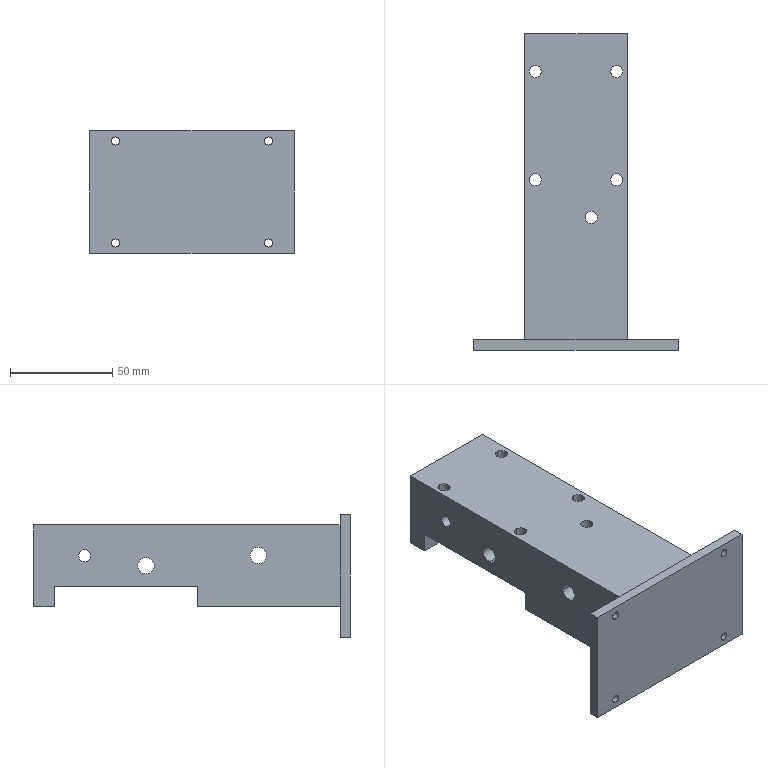Part | STEP file | Slider | 1 solid | 39 faces | box 100 x 155 x 60 mm | volume 283785 mm3 | cylinder 24 | plane 15 | commonest cylinder face diameters 6 x12 4 x8 8 x4
STEP:
#1=CARTESIAN_POINT('',(4.5,-15.,0.));
#2=VERTEX_POINT('',#1);
#3=CARTESIAN_POINT('',(10.5,-15.,0.));
#4=VERTEX_POINT('',#3);
#5=CARTESIAN_POINT('',(7.5,-15.,0.));
#6=DIRECTION('',(0.,0.,1.));
#7=DIRECTION('',(1.,0.,0.));
#8=AXIS2_PLACEMENT_3D('',#5,#6,#7);
#9=CIRCLE('',#8,3.);
#10=EDGE_CURVE('',#2,#4,#9,.T.);
#11=ORIENTED_EDGE('',*,*,#10,.F.);
#12=CARTESIAN_POINT('',(4.5,-15.,40.));
#13=VERTEX_POINT('',#12);
#14=CARTESIAN_POINT('',(4.5,-15.,-10.));
#15=DIRECTION('',(0.,0.,1.));
#16=VECTOR('',#15,1000.);
#17=LINE('',#14,#16);
#18=EDGE_CURVE('',#2,#13,#17,.T.);
#19=ORIENTED_EDGE('',*,*,#18,.T.);
#20=CARTESIAN_POINT('',(10.5,-15.,40.));
#21=VERTEX_POINT('',#20);
#22=CARTESIAN_POINT('',(7.5,-15.,40.));
#23=DIRECTION('',(0.,0.,-1.));
#24=DIRECTION('',(1.,0.,0.));
#25=AXIS2_PLACEMENT_3D('',#22,#23,#24);
#26=CIRCLE('',#25,3.);
#27=EDGE_CURVE('',#21,#13,#26,.T.);
#28=ORIENTED_EDGE('',*,*,#27,.F.);
#29=CARTESIAN_POINT('',(10.5,-15.,-10.));
#30=DIRECTION('',(0.,0.,1.));
#31=VECTOR('',#30,1000.);
#32=LINE('',#29,#31);
#33=EDGE_CURVE('',#4,#21,#32,.T.);
#34=ORIENTED_EDGE('',*,*,#33,.F.);
#35=EDGE_LOOP('',(#11,#19,#28,#34));
#36=FACE_OUTER_BOUND('',#35,.T.);
#37=CARTESIAN_POINT('',(7.5,-15.,-10.));
#38=DIRECTION('',(0.,0.,1.));
#39=DIRECTION('',(1.,0.,0.));
#40=AXIS2_PLACEMENT_3D('',#37,#38,#39);
#41=CYLINDRICAL_SURFACE('',#40,3.);
#42=ADVANCED_FACE('',(#36),#41,.F.);
#43=CARTESIAN_POINT('',(20.,53.5,40.));
#44=VERTEX_POINT('',#43);
#45=CARTESIAN_POINT('',(20.,59.5,40.));
#46=VERTEX_POINT('',#45);
#47=CARTESIAN_POINT('',(20.,56.5,40.));
#48=DIRECTION('',(0.,0.,-1.));
#49=DIRECTION('',(0.,1.,0.));
#50=AXIS2_PLACEMENT_3D('',#47,#48,#49);
#51=CIRCLE('',#50,3.);
#52=EDGE_CURVE('',#44,#46,#51,.T.);
#53=ORIENTED_EDGE('',*,*,#52,.F.);
#54=CARTESIAN_POINT('',(20.,53.5,10.));
#55=VERTEX_POINT('',#54);
#56=CARTESIAN_POINT('',(20.,53.5,60.));
#57=DIRECTION('',(0.,0.,-1.));
#58=VECTOR('',#57,1000.);
#59=LINE('',#56,#58);
#60=EDGE_CURVE('',#44,#55,#59,.T.);
#61=ORIENTED_EDGE('',*,*,#60,.T.);
#62=CARTESIAN_POINT('',(20.,59.5,10.));
#63=VERTEX_POINT('',#62);
#64=CARTESIAN_POINT('',(20.,56.5,10.));
#65=DIRECTION('',(0.,0.,1.));
#66=DIRECTION('',(0.,1.,0.));
#67=AXIS2_PLACEMENT_3D('',#64,#65,#66);
#68=CIRCLE('',#67,3.);
#69=EDGE_CURVE('',#63,#55,#68,.T.);
#70=ORIENTED_EDGE('',*,*,#69,.F.);
#71=CARTESIAN_POINT('',(20.,59.5,60.));
#72=DIRECTION('',(0.,0.,-1.));
#73=VECTOR('',#72,1000.);
#74=LINE('',#71,#73);
#75=EDGE_CURVE('',#46,#63,#74,.T.);
#76=ORIENTED_EDGE('',*,*,#75,.F.);
#77=EDGE_LOOP('',(#53,#61,#70,#76));
#78=FACE_OUTER_BOUND('',#77,.T.);
#79=CARTESIAN_POINT('',(20.,56.5,60.));
#80=DIRECTION('',(0.,0.,-1.));
#81=DIRECTION('',(0.,1.,0.));
#82=AXIS2_PLACEMENT_3D('',#79,#80,#81);
#83=CYLINDRICAL_SURFACE('',#82,3.);
#84=ADVANCED_FACE('',(#78),#83,.F.);
#85=CARTESIAN_POINT('',(-20.,53.5,40.));
#86=VERTEX_POINT('',#85);
#87=CARTESIAN_POINT('',(-20.,59.5,40.));
#88=VERTEX_POINT('',#87);
#89=CARTESIAN_POINT('',(-20.,56.5,40.));
#90=DIRECTION('',(0.,0.,-1.));
#91=DIRECTION('',(0.,1.,0.));
#92=AXIS2_PLACEMENT_3D('',#89,#90,#91);
#93=CIRCLE('',#92,3.);
#94=EDGE_CURVE('',#86,#88,#93,.T.);
#95=ORIENTED_EDGE('',*,*,#94,.F.);
#96=CARTESIAN_POINT('',(-20.,53.5,10.));
#97=VERTEX_POINT('',#96);
#98=CARTESIAN_POINT('',(-20.,53.5,60.));
#99=DIRECTION('',(0.,0.,-1.));
#100=VECTOR('',#99,1000.);
#101=LINE('',#98,#100);
#102=EDGE_CURVE('',#86,#97,#101,.T.);
#103=ORIENTED_EDGE('',*,*,#102,.T.);
#104=CARTESIAN_POINT('',(-20.,59.5,10.));
#105=VERTEX_POINT('',#104);
#106=CARTESIAN_POINT('',(-20.,56.5,10.));
#107=DIRECTION('',(0.,0.,1.));
#108=DIRECTION('',(0.,1.,0.));
#109=AXIS2_PLACEMENT_3D('',#106,#107,#108);
#110=CIRCLE('',#109,3.);
#111=EDGE_CURVE('',#105,#97,#110,.T.);
#112=ORIENTED_EDGE('',*,*,#111,.F.);
#113=CARTESIAN_POINT('',(-20.,59.5,60.));
#114=DIRECTION('',(0.,0.,-1.));
#115=VECTOR('',#114,1000.);
#116=LINE('',#113,#115);
#117=EDGE_CURVE('',#88,#105,#116,.T.);
#118=ORIENTED_EDGE('',*,*,#117,.F.);
#119=EDGE_LOOP('',(#95,#103,#112,#118));
#120=FACE_OUTER_BOUND('',#119,.T.);
#121=CARTESIAN_POINT('',(-20.,56.5,60.));
#122=DIRECTION('',(0.,0.,-1.));
#123=DIRECTION('',(0.,1.,0.));
#124=AXIS2_PLACEMENT_3D('',#121,#122,#123);
#125=CYLINDRICAL_SURFACE('',#124,3.);
#126=ADVANCED_FACE('',(#120),#125,.F.);
#127=CARTESIAN_POINT('',(20.,0.5,40.));
#128=VERTEX_POINT('',#127);
#129=CARTESIAN_POINT('',(20.,6.5,40.));
#130=VERTEX_POINT('',#129);
#131=CARTESIAN_POINT('',(20.,3.5,40.));
#132=DIRECTION('',(0.,0.,-1.));
#133=DIRECTION('',(0.,1.,0.));
#134=AXIS2_PLACEMENT_3D('',#131,#132,#133);
#135=CIRCLE('',#134,3.);
#136=EDGE_CURVE('',#128,#130,#135,.T.);
#137=ORIENTED_EDGE('',*,*,#136,.F.);
#138=CARTESIAN_POINT('',(20.,0.5,10.));
#139=VERTEX_POINT('',#138);
#140=CARTESIAN_POINT('',(20.,0.5,60.));
#141=DIRECTION('',(0.,0.,-1.));
#142=VECTOR('',#141,1000.);
#143=LINE('',#140,#142);
#144=EDGE_CURVE('',#128,#139,#143,.T.);
#145=ORIENTED_EDGE('',*,*,#144,.T.);
#146=CARTESIAN_POINT('',(20.,6.5,10.));
#147=VERTEX_POINT('',#146);
#148=CARTESIAN_POINT('',(20.,3.5,10.));
#149=DIRECTION('',(0.,0.,1.));
#150=DIRECTION('',(0.,1.,0.));
#151=AXIS2_PLACEMENT_3D('',#148,#149,#150);
#152=CIRCLE('',#151,3.);
#153=EDGE_CURVE('',#147,#139,#152,.T.);
#154=ORIENTED_EDGE('',*,*,#153,.F.);
#155=CARTESIAN_POINT('',(20.,6.5,60.));
#156=DIRECTION('',(0.,0.,-1.));
#157=VECTOR('',#156,1000.);
#158=LINE('',#155,#157);
#159=EDGE_CURVE('',#130,#147,#158,.T.);
#160=ORIENTED_EDGE('',*,*,#159,.F.);
#161=EDGE_LOOP('',(#137,#145,#154,#160));
#162=FACE_OUTER_BOUND('',#161,.T.);
#163=CARTESIAN_POINT('',(20.,3.5,60.));
#164=DIRECTION('',(0.,0.,-1.));
#165=DIRECTION('',(0.,1.,0.));
#166=AXIS2_PLACEMENT_3D('',#163,#164,#165);
#167=CYLINDRICAL_SURFACE('',#166,3.);
#168=ADVANCED_FACE('',(#162),#167,.F.);
#169=CARTESIAN_POINT('',(-20.,0.5,40.));
#170=VERTEX_POINT('',#169);
#171=CARTESIAN_POINT('',(-20.,6.5,40.));
#172=VERTEX_POINT('',#171);
#173=CARTESIAN_POINT('',(-20.,3.5,40.));
#174=DIRECTION('',(0.,0.,-1.));
#175=DIRECTION('',(0.,1.,0.));
#176=AXIS2_PLACEMENT_3D('',#173,#174,#175);
#177=CIRCLE('',#176,3.);
#178=EDGE_CURVE('',#170,#172,#177,.T.);
#179=ORIENTED_EDGE('',*,*,#178,.F.);
#180=CARTESIAN_POINT('',(-20.,0.5,10.));
#181=VERTEX_POINT('',#180);
#182=CARTESIAN_POINT('',(-20.,0.5,60.));
#183=DIRECTION('',(0.,0.,-1.));
#184=VECTOR('',#183,1000.);
#185=LINE('',#182,#184);
#186=EDGE_CURVE('',#170,#181,#185,.T.);
#187=ORIENTED_EDGE('',*,*,#186,.T.);
#188=CARTESIAN_POINT('',(-20.,6.5,10.));
#189=VERTEX_POINT('',#188);
#190=CARTESIAN_POINT('',(-20.,3.5,10.));
#191=DIRECTION('',(0.,0.,1.));
#192=DIRECTION('',(0.,1.,0.));
#193=AXIS2_PLACEMENT_3D('',#190,#191,#192);
#194=CIRCLE('',#193,3.);
#195=EDGE_CURVE('',#189,#181,#194,.T.);
#196=ORIENTED_EDGE('',*,*,#195,.F.);
#197=CARTESIAN_POINT('',(-20.,6.5,60.));
#198=DIRECTION('',(0.,0.,-1.));
#199=VECTOR('',#198,1000.);
#200=LINE('',#197,#199);
#201=EDGE_CURVE('',#172,#189,#200,.T.);
#202=ORIENTED_EDGE('',*,*,#201,.F.);
#203=EDGE_LOOP('',(#179,#187,#196,#202));
#204=FACE_OUTER_BOUND('',#203,.T.);
#205=CARTESIAN_POINT('',(-20.,3.5,60.));
#206=DIRECTION('',(0.,0.,-1.));
#207=DIRECTION('',(0.,1.,0.));
#208=AXIS2_PLACEMENT_3D('',#205,#206,#207);
#209=CYLINDRICAL_SURFACE('',#208,3.);
#210=ADVANCED_FACE('',(#204),#209,.F.);
#211=CARTESIAN_POINT('',(25.,50.,28.));
#212=VERTEX_POINT('',#211);
#213=CARTESIAN_POINT('',(25.,50.,22.));
#214=VERTEX_POINT('',#213);
#215=CARTESIAN_POINT('',(25.,50.,25.));
#216=DIRECTION('',(1.,0.,0.));
#217=DIRECTION('',(0.,0.,1.));
#218=AXIS2_PLACEMENT_3D('',#215,#216,#217);
#219=CIRCLE('',#218,3.);
#220=EDGE_CURVE('',#212,#214,#219,.T.);
#221=ORIENTED_EDGE('',*,*,#220,.T.);
#222=CARTESIAN_POINT('',(-25.,50.,22.));
#223=VERTEX_POINT('',#222);
#224=CARTESIAN_POINT('',(30.,50.,22.));
#225=DIRECTION('',(-1.,0.,0.));
#226=VECTOR('',#225,1000.);
#227=LINE('',#224,#226);
#228=EDGE_CURVE('',#214,#223,#227,.T.);
#229=ORIENTED_EDGE('',*,*,#228,.T.);
#230=CARTESIAN_POINT('',(-25.,50.,28.));
#231=VERTEX_POINT('',#230);
#232=CARTESIAN_POINT('',(-25.,50.,25.));
#233=DIRECTION('',(-1.,0.,0.));
#234=DIRECTION('',(0.,0.,1.));
#235=AXIS2_PLACEMENT_3D('',#232,#233,#234);
#236=CIRCLE('',#235,3.);
#237=EDGE_CURVE('',#223,#231,#236,.T.);
#238=ORIENTED_EDGE('',*,*,#237,.T.);
#239=CARTESIAN_POINT('',(30.,50.,28.));
#240=DIRECTION('',(-1.,0.,0.));
#241=VECTOR('',#240,1000.);
#242=LINE('',#239,#241);
#243=EDGE_CURVE('',#212,#231,#242,.T.);
#244=ORIENTED_EDGE('',*,*,#243,.F.);
#245=EDGE_LOOP('',(#221,#229,#238,#244));
#246=FACE_OUTER_BOUND('',#245,.T.);
#247=CARTESIAN_POINT('',(30.,50.,25.));
#248=DIRECTION('',(-1.,0.,0.));
#249=DIRECTION('',(0.,0.,1.));
#250=AXIS2_PLACEMENT_3D('',#247,#248,#249);
#251=CYLINDRICAL_SURFACE('',#250,3.);
#252=ADVANCED_FACE('',(#246),#251,.F.);
#253=CARTESIAN_POINT('',(25.,20.,24.));
#254=VERTEX_POINT('',#253);
#255=CARTESIAN_POINT('',(25.,20.,16.));
#256=VERTEX_POINT('',#255);
#257=CARTESIAN_POINT('',(25.,20.,20.));
#258=DIRECTION('',(1.,0.,0.));
#259=DIRECTION('',(0.,0.,1.));
#260=AXIS2_PLACEMENT_3D('',#257,#258,#259);
#261=CIRCLE('',#260,4.);
#262=EDGE_CURVE('',#254,#256,#261,.T.);
#263=ORIENTED_EDGE('',*,*,#262,.T.);
#264=CARTESIAN_POINT('',(-25.,20.,16.));
#265=VERTEX_POINT('',#264);
#266=CARTESIAN_POINT('',(50.,20.,16.));
#267=DIRECTION('',(-1.,0.,0.));
#268=VECTOR('',#267,1000.);
#269=LINE('',#266,#268);
#270=EDGE_CURVE('',#256,#265,#269,.T.);
#271=ORIENTED_EDGE('',*,*,#270,.T.);
#272=CARTESIAN_POINT('',(-25.,20.,24.));
#273=VERTEX_POINT('',#272);
#274=CARTESIAN_POINT('',(-25.,20.,20.));
#275=DIRECTION('',(-1.,0.,0.));
#276=DIRECTION('',(0.,0.,1.));
#277=AXIS2_PLACEMENT_3D('',#274,#275,#276);
#278=CIRCLE('',#277,4.);
#279=EDGE_CURVE('',#265,#273,#278,.T.);
#280=ORIENTED_EDGE('',*,*,#279,.T.);
#281=CARTESIAN_POINT('',(50.,20.,24.));
#282=DIRECTION('',(-1.,0.,0.));
#283=VECTOR('',#282,1000.);
#284=LINE('',#281,#283);
#285=EDGE_CURVE('',#254,#273,#284,.T.);
#286=ORIENTED_EDGE('',*,*,#285,.F.);
#287=EDGE_LOOP('',(#263,#271,#280,#286));
#288=FACE_OUTER_BOUND('',#287,.T.);
#289=CARTESIAN_POINT('',(50.,20.,20.));
#290=DIRECTION('',(-1.,0.,0.));
#291=DIRECTION('',(0.,0.,1.));
#292=AXIS2_PLACEMENT_3D('',#289,#290,#291);
#293=CYLINDRICAL_SURFACE('',#292,4.);
#294=ADVANCED_FACE('',(#288),#293,.F.);
#295=CARTESIAN_POINT('',(-25.,-31.,25.));
#296=VERTEX_POINT('',#295);
#297=CARTESIAN_POINT('',(-25.,-39.,25.));
#298=VERTEX_POINT('',#297);
#299=CARTESIAN_POINT('',(-25.,-35.,25.));
#300=DIRECTION('',(-1.,0.,0.));
#301=DIRECTION('',(0.,1.,0.));
#302=AXIS2_PLACEMENT_3D('',#299,#300,#301);
#303=CIRCLE('',#302,4.);
#304=EDGE_CURVE('',#296,#298,#303,.T.);
#305=ORIENTED_EDGE('',*,*,#304,.T.);
#306=CARTESIAN_POINT('',(25.,-39.,25.));
#307=VERTEX_POINT('',#306);
#308=CARTESIAN_POINT('',(-50.,-39.,25.));
#309=DIRECTION('',(1.,0.,0.));
#310=VECTOR('',#309,1000.);
#311=LINE('',#308,#310);
#312=EDGE_CURVE('',#298,#307,#311,.T.);
#313=ORIENTED_EDGE('',*,*,#312,.T.);
#314=CARTESIAN_POINT('',(25.,-31.,25.));
#315=VERTEX_POINT('',#314);
#316=CARTESIAN_POINT('',(25.,-35.,25.));
#317=DIRECTION('',(1.,0.,0.));
#318=DIRECTION('',(0.,1.,0.));
#319=AXIS2_PLACEMENT_3D('',#316,#317,#318);
#320=CIRCLE('',#319,4.);
#321=EDGE_CURVE('',#307,#315,#320,.T.);
#322=ORIENTED_EDGE('',*,*,#321,.T.);
#323=CARTESIAN_POINT('',(-50.,-31.,25.));
#324=DIRECTION('',(1.,0.,0.));
#325=VECTOR('',#324,1000.);
#326=LINE('',#323,#325);
#327=EDGE_CURVE('',#296,#315,#326,.T.);
#328=ORIENTED_EDGE('',*,*,#327,.F.);
#329=EDGE_LOOP('',(#305,#313,#322,#328));
#330=FACE_OUTER_BOUND('',#329,.T.);
#331=CARTESIAN_POINT('',(-50.,-35.,25.));
#332=DIRECTION('',(1.,0.,0.));
#333=DIRECTION('',(0.,1.,0.));
#334=AXIS2_PLACEMENT_3D('',#331,#332,#333);
#335=CYLINDRICAL_SURFACE('',#334,4.);
#336=ADVANCED_FACE('',(#330),#335,.F.);
#337=CARTESIAN_POINT('',(-37.5,-80.,-12.));
#338=VERTEX_POINT('',#337);
#339=CARTESIAN_POINT('',(-37.5,-80.,-8.));
#340=VERTEX_POINT('',#339);
#341=CARTESIAN_POINT('',(-37.5,-80.,-10.));
#342=DIRECTION('',(0.,1.,0.));
#343=DIRECTION('',(0.,0.,1.));
#344=AXIS2_PLACEMENT_3D('',#341,#342,#343);
#345=CIRCLE('',#344,2.);
#346=EDGE_CURVE('',#338,#340,#345,.T.);
#347=ORIENTED_EDGE('',*,*,#346,.F.);
#348=CARTESIAN_POINT('',(-37.5,-75.,-12.));
#349=VERTEX_POINT('',#348);
#350=CARTESIAN_POINT('',(-37.5,-80.,-12.));
#351=DIRECTION('',(0.,1.,0.));
#352=VECTOR('',#351,1000.);
#353=LINE('',#350,#352);
#354=EDGE_CURVE('',#338,#349,#353,.T.);
#355=ORIENTED_EDGE('',*,*,#354,.T.);
#356=CARTESIAN_POINT('',(-37.5,-75.,-8.));
#357=VERTEX_POINT('',#356);
#358=CARTESIAN_POINT('',(-37.5,-75.,-10.));
#359=DIRECTION('',(0.,1.,0.));
#360=DIRECTION('',(0.,0.,1.));
#361=AXIS2_PLACEMENT_3D('',#358,#359,#360);
#362=CIRCLE('',#361,2.);
#363=EDGE_CURVE('',#349,#357,#362,.T.);
#364=ORIENTED_EDGE('',*,*,#363,.T.);
#365=CARTESIAN_POINT('',(-37.5,-80.,-8.));
#366=DIRECTION('',(0.,1.,0.));
#367=VECTOR('',#366,1000.);
#368=LINE('',#365,#367);
#369=EDGE_CURVE('',#340,#357,#368,.T.);
#370=ORIENTED_EDGE('',*,*,#369,.F.);
#371=EDGE_LOOP('',(#347,#355,#364,#370));
#372=FACE_OUTER_BOUND('',#371,.T.);
#373=CARTESIAN_POINT('',(-37.5,-80.,-10.));
#374=DIRECTION('',(0.,1.,0.));
#375=DIRECTION('',(0.,0.,1.));
#376=AXIS2_PLACEMENT_3D('',#373,#374,#375);
#377=CYLINDRICAL_SURFACE('',#376,2.);
#378=ADVANCED_FACE('',(#372),#377,.F.);
#379=CARTESIAN_POINT('',(37.5,-80.,38.));
#380=VERTEX_POINT('',#379);
#381=CARTESIAN_POINT('',(37.5,-80.,42.));
#382=VERTEX_POINT('',#381);
#383=CARTESIAN_POINT('',(37.5,-80.,40.));
#384=DIRECTION('',(0.,1.,0.));
#385=DIRECTION('',(0.,0.,1.));
#386=AXIS2_PLACEMENT_3D('',#383,#384,#385);
#387=CIRCLE('',#386,2.);
#388=EDGE_CURVE('',#380,#382,#387,.T.);
#389=ORIENTED_EDGE('',*,*,#388,.F.);
#390=CARTESIAN_POINT('',(37.5,-75.,38.));
#391=VERTEX_POINT('',#390);
#392=CARTESIAN_POINT('',(37.5,-80.,38.));
#393=DIRECTION('',(0.,1.,0.));
#394=VECTOR('',#393,1000.);
#395=LINE('',#392,#394);
#396=EDGE_CURVE('',#380,#391,#395,.T.);
#397=ORIENTED_EDGE('',*,*,#396,.T.);
#398=CARTESIAN_POINT('',(37.5,-75.,42.));
#399=VERTEX_POINT('',#398);
#400=CARTESIAN_POINT('',(37.5,-75.,40.));
#401=DIRECTION('',(0.,1.,0.));
#402=DIRECTION('',(0.,0.,1.));
#403=AXIS2_PLACEMENT_3D('',#400,#401,#402);
#404=CIRCLE('',#403,2.);
#405=EDGE_CURVE('',#391,#399,#404,.T.);
#406=ORIENTED_EDGE('',*,*,#405,.T.);
#407=CARTESIAN_POINT('',(37.5,-80.,42.));
#408=DIRECTION('',(0.,1.,0.));
#409=VECTOR('',#408,1000.);
#410=LINE('',#407,#409);
#411=EDGE_CURVE('',#382,#399,#410,.T.);
#412=ORIENTED_EDGE('',*,*,#411,.F.);
#413=EDGE_LOOP('',(#389,#397,#406,#412));
#414=FACE_OUTER_BOUND('',#413,.T.);
#415=CARTESIAN_POINT('',(37.5,-80.,40.));
#416=DIRECTION('',(0.,1.,0.));
#417=DIRECTION('',(0.,0.,1.));
#418=AXIS2_PLACEMENT_3D('',#415,#416,#417);
#419=CYLINDRICAL_SURFACE('',#418,2.);
#420=ADVANCED_FACE('',(#414),#419,.F.);
#421=CARTESIAN_POINT('',(-37.5,-80.,38.));
#422=VERTEX_POINT('',#421);
#423=CARTESIAN_POINT('',(-37.5,-80.,42.));
#424=VERTEX_POINT('',#423);
#425=CARTESIAN_POINT('',(-37.5,-80.,40.));
#426=DIRECTION('',(0.,1.,0.));
#427=DIRECTION('',(0.,0.,1.));
#428=AXIS2_PLACEMENT_3D('',#425,#426,#427);
#429=CIRCLE('',#428,2.);
#430=EDGE_CURVE('',#422,#424,#429,.T.);
#431=ORIENTED_EDGE('',*,*,#430,.F.);
#432=CARTESIAN_POINT('',(-37.5,-75.,38.));
#433=VERTEX_POINT('',#432);
#434=CARTESIAN_POINT('',(-37.5,-80.,38.));
#435=DIRECTION('',(0.,1.,0.));
#436=VECTOR('',#435,1000.);
#437=LINE('',#434,#436);
#438=EDGE_CURVE('',#422,#433,#437,.T.);
#439=ORIENTED_EDGE('',*,*,#438,.T.);
#440=CARTESIAN_POINT('',(-37.5,-75.,42.));
#441=VERTEX_POINT('',#440);
#442=CARTESIAN_POINT('',(-37.5,-75.,40.));
#443=DIRECTION('',(0.,1.,0.));
#444=DIRECTION('',(0.,0.,1.));
#445=AXIS2_PLACEMENT_3D('',#442,#443,#444);
#446=CIRCLE('',#445,2.);
#447=EDGE_CURVE('',#433,#441,#446,.T.);
#448=ORIENTED_EDGE('',*,*,#447,.T.);
#449=CARTESIAN_POINT('',(-37.5,-80.,42.));
#450=DIRECTION('',(0.,1.,0.));
#451=VECTOR('',#450,1000.);
#452=LINE('',#449,#451);
#453=EDGE_CURVE('',#424,#441,#452,.T.);
#454=ORIENTED_EDGE('',*,*,#453,.F.);
#455=EDGE_LOOP('',(#431,#439,#448,#454));
#456=FACE_OUTER_BOUND('',#455,.T.);
#457=CARTESIAN_POINT('',(-37.5,-80.,40.));
#458=DIRECTION('',(0.,1.,0.));
#459=DIRECTION('',(0.,0.,1.));
#460=AXIS2_PLACEMENT_3D('',#457,#458,#459);
#461=CYLINDRICAL_SURFACE('',#460,2.);
#462=ADVANCED_FACE('',(#456),#461,.F.);
#463=CARTESIAN_POINT('',(37.5,-80.,-12.));
#464=VERTEX_POINT('',#463);
#465=CARTESIAN_POINT('',(37.5,-80.,-8.));
#466=VERTEX_POINT('',#465);
#467=CARTESIAN_POINT('',(37.5,-80.,-10.));
#468=DIRECTION('',(0.,1.,0.));
#469=DIRECTION('',(0.,0.,1.));
#470=AXIS2_PLACEMENT_3D('',#467,#468,#469);
#471=CIRCLE('',#470,2.);
#472=EDGE_CURVE('',#464,#466,#471,.T.);
#473=ORIENTED_EDGE('',*,*,#472,.F.);
#474=CARTESIAN_POINT('',(37.5,-75.,-12.));
#475=VERTEX_POINT('',#474);
#476=CARTESIAN_POINT('',(37.5,-80.,-12.));
#477=DIRECTION('',(0.,1.,0.));
#478=VECTOR('',#477,1000.);
#479=LINE('',#476,#478);
#480=EDGE_CURVE('',#464,#475,#479,.T.);
#481=ORIENTED_EDGE('',*,*,#480,.T.);
#482=CARTESIAN_POINT('',(37.5,-75.,-8.));
#483=VERTEX_POINT('',#482);
#484=CARTESIAN_POINT('',(37.5,-75.,-10.));
#485=DIRECTION('',(0.,1.,0.));
#486=DIRECTION('',(0.,0.,1.));
#487=AXIS2_PLACEMENT_3D('',#484,#485,#486);
#488=CIRCLE('',#487,2.);
#489=EDGE_CURVE('',#475,#483,#488,.T.);
#490=ORIENTED_EDGE('',*,*,#489,.T.);
#491=CARTESIAN_POINT('',(37.5,-80.,-8.));
#492=DIRECTION('',(0.,1.,0.));
#493=VECTOR('',#492,1000.);
#494=LINE('',#491,#493);
#495=EDGE_CURVE('',#466,#483,#494,.T.);
#496=ORIENTED_EDGE('',*,*,#495,.F.);
#497=EDGE_LOOP('',(#473,#481,#490,#496));
#498=FACE_OUTER_BOUND('',#497,.T.);
#499=CARTESIAN_POINT('',(37.5,-80.,-10.));
#500=DIRECTION('',(0.,1.,0.));
#501=DIRECTION('',(0.,0.,1.));
#502=AXIS2_PLACEMENT_3D('',#499,#500,#501);
#503=CYLINDRICAL_SURFACE('',#502,2.);
#504=ADVANCED_FACE('',(#498),#503,.F.);
#505=CARTESIAN_POINT('',(25.,-75.,40.));
#506=VERTEX_POINT('',#505);
#507=CARTESIAN_POINT('',(25.,75.,40.));
#508=VERTEX_POINT('',#507);
#509=CARTESIAN_POINT('',(25.,-75.,40.));
#510=DIRECTION('',(0.,1.,0.));
#511=VECTOR('',#510,1000.);
#512=LINE('',#509,#511);
#513=EDGE_CURVE('',#506,#508,#512,.T.);
#514=ORIENTED_EDGE('',*,*,#513,.T.);
#515=CARTESIAN_POINT('',(-25.,75.,40.));
#516=VERTEX_POINT('',#515);
#517=CARTESIAN_POINT('',(-25.,75.,40.));
#518=DIRECTION('',(-1.,0.,0.));
#519=VECTOR('',#518,1000.);
#520=LINE('',#517,#519);
#521=EDGE_CURVE('',#508,#516,#520,.T.);
#522=ORIENTED_EDGE('',*,*,#521,.T.);
#523=CARTESIAN_POINT('',(-25.,-75.,40.));
#524=VERTEX_POINT('',#523);
#525=CARTESIAN_POINT('',(-25.,-75.,40.));
#526=DIRECTION('',(0.,-1.,0.));
#527=VECTOR('',#526,1000.);
#528=LINE('',#525,#527);
#529=EDGE_CURVE('',#516,#524,#528,.T.);
#530=ORIENTED_EDGE('',*,*,#529,.T.);
#531=CARTESIAN_POINT('',(-25.,-75.,40.));
#532=DIRECTION('',(1.,0.,0.));
#533=VECTOR('',#532,1000.);
#534=LINE('',#531,#533);
#535=EDGE_CURVE('',#524,#506,#534,.T.);
#536=ORIENTED_EDGE('',*,*,#535,.T.);
#537=EDGE_LOOP('',(#514,#522,#530,#536));
#538=FACE_OUTER_BOUND('',#537,.T.);
#539=ORIENTED_EDGE('',*,*,#27,.T.);
#540=CARTESIAN_POINT('',(7.5,-15.,40.));
#541=DIRECTION('',(0.,0.,-1.));
#542=DIRECTION('',(1.,0.,0.));
#543=AXIS2_PLACEMENT_3D('',#540,#541,#542);
#544=CIRCLE('',#543,3.);
#545=EDGE_CURVE('',#13,#21,#544,.T.);
#546=ORIENTED_EDGE('',*,*,#545,.T.);
#547=EDGE_LOOP('',(#539,#546));
#548=FACE_BOUND('',#547,.T.);
#549=CARTESIAN_POINT('',(20.,56.5,40.));
#550=DIRECTION('',(0.,0.,-1.));
#551=DIRECTION('',(0.,1.,0.));
#552=AXIS2_PLACEMENT_3D('',#549,#550,#551);
#553=CIRCLE('',#552,3.);
#554=EDGE_CURVE('',#46,#44,#553,.T.);
#555=ORIENTED_EDGE('',*,*,#554,.T.);
#556=ORIENTED_EDGE('',*,*,#52,.T.);
#557=EDGE_LOOP('',(#555,#556));
#558=FACE_BOUND('',#557,.T.);
#559=CARTESIAN_POINT('',(-20.,56.5,40.));
#560=DIRECTION('',(0.,0.,-1.));
#561=DIRECTION('',(0.,1.,0.));
#562=AXIS2_PLACEMENT_3D('',#559,#560,#561);
#563=CIRCLE('',#562,3.);
#564=EDGE_CURVE('',#88,#86,#563,.T.);
#565=ORIENTED_EDGE('',*,*,#564,.T.);
#566=ORIENTED_EDGE('',*,*,#94,.T.);
#567=EDGE_LOOP('',(#565,#566));
#568=FACE_BOUND('',#567,.T.);
#569=CARTESIAN_POINT('',(20.,3.5,40.));
#570=DIRECTION('',(0.,0.,-1.));
#571=DIRECTION('',(0.,1.,0.));
#572=AXIS2_PLACEMENT_3D('',#569,#570,#571);
#573=CIRCLE('',#572,3.);
#574=EDGE_CURVE('',#130,#128,#573,.T.);
#575=ORIENTED_EDGE('',*,*,#574,.T.);
#576=ORIENTED_EDGE('',*,*,#136,.T.);
#577=EDGE_LOOP('',(#575,#576));
#578=FACE_BOUND('',#577,.T.);
#579=CARTESIAN_POINT('',(-20.,3.5,40.));
#580=DIRECTION('',(0.,0.,-1.));
#581=DIRECTION('',(0.,1.,0.));
#582=AXIS2_PLACEMENT_3D('',#579,#580,#581);
#583=CIRCLE('',#582,3.);
#584=EDGE_CURVE('',#172,#170,#583,.T.);
#585=ORIENTED_EDGE('',*,*,#584,.T.);
#586=ORIENTED_EDGE('',*,*,#178,.T.);
#587=EDGE_LOOP('',(#585,#586));
#588=FACE_BOUND('',#587,.T.);
#589=CARTESIAN_POINT('',(-25.,-75.,40.));
#590=DIRECTION('',(0.,0.,1.));
#591=DIRECTION('',(1.,0.,0.));
#592=AXIS2_PLACEMENT_3D('',#589,#590,#591);
#593=PLANE('',#592);
#594=ADVANCED_FACE('',(#538,#548,#558,#568,#578,#588),#593,.T.);
#595=CARTESIAN_POINT('',(-25.,75.,0.));
#596=VERTEX_POINT('',#595);
#597=CARTESIAN_POINT('',(-25.,75.,40.));
#598=DIRECTION('',(0.,0.,-1.));
#599=VECTOR('',#598,1000.);
#600=LINE('',#597,#599);
#601=EDGE_CURVE('',#516,#596,#600,.T.);
#602=ORIENTED_EDGE('',*,*,#601,.F.);
#603=ORIENTED_EDGE('',*,*,#521,.F.);
#604=CARTESIAN_POINT('',(25.,75.,0.));
#605=VERTEX_POINT('',#604);
#606=CARTESIAN_POINT('',(25.,75.,40.));
#607=DIRECTION('',(0.,0.,1.));
#608=VECTOR('',#607,1000.);
#609=LINE('',#606,#608);
#610=EDGE_CURVE('',#605,#508,#609,.T.);
#611=ORIENTED_EDGE('',*,*,#610,.F.);
#612=CARTESIAN_POINT('',(-25.,75.,0.));
#613=DIRECTION('',(1.,0.,0.));
#614=VECTOR('',#613,1000.);
#615=LINE('',#612,#614);
#616=EDGE_CURVE('',#596,#605,#615,.T.);
#617=ORIENTED_EDGE('',*,*,#616,.F.);
#618=EDGE_LOOP('',(#602,#603,#611,#617));
#619=FACE_OUTER_BOUND('',#618,.T.);
#620=CARTESIAN_POINT('',(-25.,75.,40.));
#621=DIRECTION('',(0.,-1.,0.));
#622=DIRECTION('',(0.,0.,-1.));
#623=AXIS2_PLACEMENT_3D('',#620,#621,#622);
#624=PLANE('',#623);
#625=ADVANCED_FACE('',(#619),#624,.F.);
#626=CARTESIAN_POINT('',(25.,65.,0.));
#627=VERTEX_POINT('',#626);
#628=CARTESIAN_POINT('',(25.,65.,10.));
#629=VERTEX_POINT('',#628);
#630=CARTESIAN_POINT('',(25.,65.,40.));
#631=DIRECTION('',(0.,0.,1.));
#632=VECTOR('',#631,1000.);
#633=LINE('',#630,#632);
#634=EDGE_CURVE('',#627,#629,#633,.T.);
#635=ORIENTED_EDGE('',*,*,#634,.F.);
#636=CARTESIAN_POINT('',(25.,75.,0.));
#637=DIRECTION('',(0.,-1.,0.));
#638=VECTOR('',#637,1000.);
#639=LINE('',#636,#638);
#640=EDGE_CURVE('',#605,#627,#639,.T.);
#641=ORIENTED_EDGE('',*,*,#640,.F.);
#642=ORIENTED_EDGE('',*,*,#610,.T.);
#643=ORIENTED_EDGE('',*,*,#513,.F.);
#644=CARTESIAN_POINT('',(25.,-75.,0.));
#645=VERTEX_POINT('',#644);
#646=CARTESIAN_POINT('',(25.,-75.,40.));
#647=DIRECTION('',(0.,0.,1.));
#648=VECTOR('',#647,1000.);
#649=LINE('',#646,#648);
#650=EDGE_CURVE('',#645,#506,#649,.T.);
#651=ORIENTED_EDGE('',*,*,#650,.F.);
#652=CARTESIAN_POINT('',(25.,-5.,0.));
#653=VERTEX_POINT('',#652);
#654=CARTESIAN_POINT('',(25.,75.,0.));
#655=DIRECTION('',(0.,-1.,0.));
#656=VECTOR('',#655,1000.);
#657=LINE('',#654,#656);
#658=EDGE_CURVE('',#653,#645,#657,.T.);
#659=ORIENTED_EDGE('',*,*,#658,.F.);
#660=CARTESIAN_POINT('',(25.,-5.,10.));
#661=VERTEX_POINT('',#660);
#662=CARTESIAN_POINT('',(25.,-5.,40.));
#663=DIRECTION('',(0.,0.,-1.));
#664=VECTOR('',#663,1000.);
#665=LINE('',#662,#664);
#666=EDGE_CURVE('',#661,#653,#665,.T.);
#667=ORIENTED_EDGE('',*,*,#666,.F.);
#668=CARTESIAN_POINT('',(25.,75.,10.));
#669=DIRECTION('',(0.,-1.,0.));
#670=VECTOR('',#669,1000.);
#671=LINE('',#668,#670);
#672=EDGE_CURVE('',#629,#661,#671,.T.);
#673=ORIENTED_EDGE('',*,*,#672,.F.);
#674=EDGE_LOOP('',(#635,#641,#642,#643,#651,#659,#667,#673));
#675=FACE_OUTER_BOUND('',#674,.T.);
#676=ORIENTED_EDGE('',*,*,#220,.F.);
#677=CARTESIAN_POINT('',(25.,50.,25.));
#678=DIRECTION('',(1.,0.,0.));
#679=DIRECTION('',(0.,0.,1.));
#680=AXIS2_PLACEMENT_3D('',#677,#678,#679);
#681=CIRCLE('',#680,3.);
#682=EDGE_CURVE('',#214,#212,#681,.T.);
#683=ORIENTED_EDGE('',*,*,#682,.F.);
#684=EDGE_LOOP('',(#676,#683));
#685=FACE_BOUND('',#684,.T.);
#686=ORIENTED_EDGE('',*,*,#262,.F.);
#687=CARTESIAN_POINT('',(25.,20.,20.));
#688=DIRECTION('',(1.,0.,0.));
#689=DIRECTION('',(0.,0.,1.));
#690=AXIS2_PLACEMENT_3D('',#687,#688,#689);
#691=CIRCLE('',#690,4.);
#692=EDGE_CURVE('',#256,#254,#691,.T.);
#693=ORIENTED_EDGE('',*,*,#692,.F.);
#694=EDGE_LOOP('',(#686,#693));
#695=FACE_BOUND('',#694,.T.);
#696=CARTESIAN_POINT('',(25.,-35.,25.));
#697=DIRECTION('',(1.,0.,0.));
#698=DIRECTION('',(0.,1.,0.));
#699=AXIS2_PLACEMENT_3D('',#696,#697,#698);
#700=CIRCLE('',#699,4.);
#701=EDGE_CURVE('',#315,#307,#700,.T.);
#702=ORIENTED_EDGE('',*,*,#701,.F.);
#703=ORIENTED_EDGE('',*,*,#321,.F.);
#704=EDGE_LOOP('',(#702,#703));
#705=FACE_BOUND('',#704,.T.);
#706=CARTESIAN_POINT('',(25.,75.,40.));
#707=DIRECTION('',(-1.,0.,0.));
#708=DIRECTION('',(0.,-1.,0.));
#709=AXIS2_PLACEMENT_3D('',#706,#707,#708);
#710=PLANE('',#709);
#711=ADVANCED_FACE('',(#675,#685,#695,#705),#710,.F.);
#712=CARTESIAN_POINT('',(-37.5,-75.,-10.));
#713=DIRECTION('',(0.,1.,0.));
#714=DIRECTION('',(0.,0.,1.));
#715=AXIS2_PLACEMENT_3D('',#712,#713,#714);
#716=CIRCLE('',#715,2.);
#717=EDGE_CURVE('',#357,#349,#716,.T.);
#718=ORIENTED_EDGE('',*,*,#717,.F.);
#719=ORIENTED_EDGE('',*,*,#363,.F.);
#720=EDGE_LOOP('',(#718,#719));
#721=FACE_BOUND('',#720,.T.);
#722=CARTESIAN_POINT('',(37.5,-75.,40.));
#723=DIRECTION('',(0.,1.,0.));
#724=DIRECTION('',(0.,0.,1.));
#725=AXIS2_PLACEMENT_3D('',#722,#723,#724);
#726=CIRCLE('',#725,2.);
#727=EDGE_CURVE('',#399,#391,#726,.T.);
#728=ORIENTED_EDGE('',*,*,#727,.F.);
#729=ORIENTED_EDGE('',*,*,#405,.F.);
#730=EDGE_LOOP('',(#728,#729));
#731=FACE_BOUND('',#730,.T.);
#732=CARTESIAN_POINT('',(50.,-75.,45.));
#733=VERTEX_POINT('',#732);
#734=CARTESIAN_POINT('',(-50.,-75.,45.));
#735=VERTEX_POINT('',#734);
#736=CARTESIAN_POINT('',(-50.,-75.,45.));
#737=DIRECTION('',(-1.,0.,0.));
#738=VECTOR('',#737,1000.);
#739=LINE('',#736,#738);
#740=EDGE_CURVE('',#733,#735,#739,.T.);
#741=ORIENTED_EDGE('',*,*,#740,.F.);
#742=CARTESIAN_POINT('',(50.,-75.,-15.));
#743=VERTEX_POINT('',#742);
#744=CARTESIAN_POINT('',(50.,-75.,45.));
#745=DIRECTION('',(0.,0.,1.));
#746=VECTOR('',#745,1000.);
#747=LINE('',#744,#746);
#748=EDGE_CURVE('',#743,#733,#747,.T.);
#749=ORIENTED_EDGE('',*,*,#748,.F.);
#750=CARTESIAN_POINT('',(-50.,-75.,-15.));
#751=VERTEX_POINT('',#750);
#752=CARTESIAN_POINT('',(-50.,-75.,-15.));
#753=DIRECTION('',(1.,0.,0.));
#754=VECTOR('',#753,1000.);
#755=LINE('',#752,#754);
#756=EDGE_CURVE('',#751,#743,#755,.T.);
#757=ORIENTED_EDGE('',*,*,#756,.F.);
#758=CARTESIAN_POINT('',(-50.,-75.,45.));
#759=DIRECTION('',(0.,0.,-1.));
#760=VECTOR('',#759,1000.);
#761=LINE('',#758,#760);
#762=EDGE_CURVE('',#735,#751,#761,.T.);
#763=ORIENTED_EDGE('',*,*,#762,.F.);
#764=EDGE_LOOP('',(#741,#749,#757,#763));
#765=FACE_OUTER_BOUND('',#764,.T.);
#766=CARTESIAN_POINT('',(-37.5,-75.,40.));
#767=DIRECTION('',(0.,1.,0.));
#768=DIRECTION('',(0.,0.,1.));
#769=AXIS2_PLACEMENT_3D('',#766,#767,#768);
#770=CIRCLE('',#769,2.);
#771=EDGE_CURVE('',#441,#433,#770,.T.);
#772=ORIENTED_EDGE('',*,*,#771,.F.);
#773=ORIENTED_EDGE('',*,*,#447,.F.);
#774=EDGE_LOOP('',(#772,#773));
#775=FACE_BOUND('',#774,.T.);
#776=CARTESIAN_POINT('',(37.5,-75.,-10.));
#777=DIRECTION('',(0.,1.,0.));
#778=DIRECTION('',(0.,0.,1.));
#779=AXIS2_PLACEMENT_3D('',#776,#777,#778);
#780=CIRCLE('',#779,2.);
#781=EDGE_CURVE('',#483,#475,#780,.T.);
#782=ORIENTED_EDGE('',*,*,#781,.F.);
#783=ORIENTED_EDGE('',*,*,#489,.F.);
#784=EDGE_LOOP('',(#782,#783));
#785=FACE_BOUND('',#784,.T.);
#786=CARTESIAN_POINT('',(-25.,-75.,0.));
#787=VERTEX_POINT('',#786);
#788=CARTESIAN_POINT('',(-25.,-75.,45.));
#789=DIRECTION('',(0.,0.,1.));
#790=VECTOR('',#789,1000.);
#791=LINE('',#788,#790);
#792=EDGE_CURVE('',#787,#524,#791,.T.);
#793=ORIENTED_EDGE('',*,*,#792,.F.);
#794=CARTESIAN_POINT('',(-50.,-75.,0.));
#795=DIRECTION('',(-1.,0.,0.));
#796=VECTOR('',#795,1000.);
#797=LINE('',#794,#796);
#798=EDGE_CURVE('',#645,#787,#797,.T.);
#799=ORIENTED_EDGE('',*,*,#798,.F.);
#800=ORIENTED_EDGE('',*,*,#650,.T.);
#801=ORIENTED_EDGE('',*,*,#535,.F.);
#802=EDGE_LOOP('',(#793,#799,#800,#801));
#803=FACE_BOUND('',#802,.T.);
#804=CARTESIAN_POINT('',(-50.,-75.,45.));
#805=DIRECTION('',(0.,-1.,0.));
#806=DIRECTION('',(0.,0.,-1.));
#807=AXIS2_PLACEMENT_3D('',#804,#805,#806);
#808=PLANE('',#807);
#809=ADVANCED_FACE('',(#721,#731,#765,#775,#785,#803),#808,.F.);
#810=CARTESIAN_POINT('',(-25.,65.,10.));
#811=VERTEX_POINT('',#810);
#812=CARTESIAN_POINT('',(-25.,65.,0.));
#813=VERTEX_POINT('',#812);
#814=CARTESIAN_POINT('',(-25.,65.,40.));
#815=DIRECTION('',(0.,0.,-1.));
#816=VECTOR('',#815,1000.);
#817=LINE('',#814,#816);
#818=EDGE_CURVE('',#811,#813,#817,.T.);
#819=ORIENTED_EDGE('',*,*,#818,.F.);
#820=CARTESIAN_POINT('',(-25.,-5.,10.));
#821=VERTEX_POINT('',#820);
#822=CARTESIAN_POINT('',(-25.,75.,10.));
#823=DIRECTION('',(0.,1.,0.));
#824=VECTOR('',#823,1000.);
#825=LINE('',#822,#824);
#826=EDGE_CURVE('',#821,#811,#825,.T.);
#827=ORIENTED_EDGE('',*,*,#826,.F.);
#828=CARTESIAN_POINT('',(-25.,-5.,0.));
#829=VERTEX_POINT('',#828);
#830=CARTESIAN_POINT('',(-25.,-5.,40.));
#831=DIRECTION('',(0.,0.,1.));
#832=VECTOR('',#831,1000.);
#833=LINE('',#830,#832);
#834=EDGE_CURVE('',#829,#821,#833,.T.);
#835=ORIENTED_EDGE('',*,*,#834,.F.);
#836=CARTESIAN_POINT('',(-25.,75.,0.));
#837=DIRECTION('',(0.,1.,0.));
#838=VECTOR('',#837,1000.);
#839=LINE('',#836,#838);
#840=EDGE_CURVE('',#787,#829,#839,.T.);
#841=ORIENTED_EDGE('',*,*,#840,.F.);
#842=ORIENTED_EDGE('',*,*,#792,.T.);
#843=ORIENTED_EDGE('',*,*,#529,.F.);
#844=ORIENTED_EDGE('',*,*,#601,.T.);
#845=CARTESIAN_POINT('',(-25.,75.,0.));
#846=DIRECTION('',(0.,1.,0.));
#847=VECTOR('',#846,1000.);
#848=LINE('',#845,#847);
#849=EDGE_CURVE('',#813,#596,#848,.T.);
#850=ORIENTED_EDGE('',*,*,#849,.F.);
#851=EDGE_LOOP('',(#819,#827,#835,#841,#842,#843,#844,#850));
#852=FACE_OUTER_BOUND('',#851,.T.);
#853=CARTESIAN_POINT('',(-25.,50.,25.));
#854=DIRECTION('',(-1.,0.,0.));
#855=DIRECTION('',(0.,0.,1.));
#856=AXIS2_PLACEMENT_3D('',#853,#854,#855);
#857=CIRCLE('',#856,3.);
#858=EDGE_CURVE('',#231,#223,#857,.T.);
#859=ORIENTED_EDGE('',*,*,#858,.F.);
#860=ORIENTED_EDGE('',*,*,#237,.F.);
#861=EDGE_LOOP('',(#859,#860));
#862=FACE_BOUND('',#861,.T.);
#863=CARTESIAN_POINT('',(-25.,20.,20.));
#864=DIRECTION('',(-1.,0.,0.));
#865=DIRECTION('',(0.,0.,1.));
#866=AXIS2_PLACEMENT_3D('',#863,#864,#865);
#867=CIRCLE('',#866,4.);
#868=EDGE_CURVE('',#273,#265,#867,.T.);
#869=ORIENTED_EDGE('',*,*,#868,.F.);
#870=ORIENTED_EDGE('',*,*,#279,.F.);
#871=EDGE_LOOP('',(#869,#870));
#872=FACE_BOUND('',#871,.T.);
#873=ORIENTED_EDGE('',*,*,#304,.F.);
#874=CARTESIAN_POINT('',(-25.,-35.,25.));
#875=DIRECTION('',(-1.,0.,0.));
#876=DIRECTION('',(0.,1.,0.));
#877=AXIS2_PLACEMENT_3D('',#874,#875,#876);
#878=CIRCLE('',#877,4.);
#879=EDGE_CURVE('',#298,#296,#878,.T.);
#880=ORIENTED_EDGE('',*,*,#879,.F.);
#881=EDGE_LOOP('',(#873,#880));
#882=FACE_BOUND('',#881,.T.);
#883=CARTESIAN_POINT('',(-25.,75.,40.));
#884=DIRECTION('',(1.,0.,0.));
#885=DIRECTION('',(0.,1.,0.));
#886=AXIS2_PLACEMENT_3D('',#883,#884,#885);
#887=PLANE('',#886);
#888=ADVANCED_FACE('',(#852,#862,#872,#882),#887,.F.);
#889=ORIENTED_EDGE('',*,*,#18,.F.);
#890=CARTESIAN_POINT('',(7.5,-15.,0.));
#891=DIRECTION('',(0.,0.,1.));
#892=DIRECTION('',(1.,0.,0.));
#893=AXIS2_PLACEMENT_3D('',#890,#891,#892);
#894=CIRCLE('',#893,3.);
#895=EDGE_CURVE('',#4,#2,#894,.T.);
#896=ORIENTED_EDGE('',*,*,#895,.F.);
#897=ORIENTED_EDGE('',*,*,#33,.T.);
#898=ORIENTED_EDGE('',*,*,#545,.F.);
#899=EDGE_LOOP('',(#889,#896,#897,#898));
#900=FACE_OUTER_BOUND('',#899,.T.);
#901=CARTESIAN_POINT('',(7.5,-15.,-10.));
#902=DIRECTION('',(0.,0.,1.));
#903=DIRECTION('',(1.,0.,0.));
#904=AXIS2_PLACEMENT_3D('',#901,#902,#903);
#905=CYLINDRICAL_SURFACE('',#904,3.);
#906=ADVANCED_FACE('',(#900),#905,.F.);
#907=ORIENTED_EDGE('',*,*,#60,.F.);
#908=ORIENTED_EDGE('',*,*,#554,.F.);
#909=ORIENTED_EDGE('',*,*,#75,.T.);
#910=CARTESIAN_POINT('',(20.,56.5,10.));
#911=DIRECTION('',(0.,0.,1.));
#912=DIRECTION('',(0.,1.,0.));
#913=AXIS2_PLACEMENT_3D('',#910,#911,#912);
#914=CIRCLE('',#913,3.);
#915=EDGE_CURVE('',#55,#63,#914,.T.);
#916=ORIENTED_EDGE('',*,*,#915,.F.);
#917=EDGE_LOOP('',(#907,#908,#909,#916));
#918=FACE_OUTER_BOUND('',#917,.T.);
#919=CARTESIAN_POINT('',(20.,56.5,60.));
#920=DIRECTION('',(0.,0.,-1.));
#921=DIRECTION('',(0.,1.,0.));
#922=AXIS2_PLACEMENT_3D('',#919,#920,#921);
#923=CYLINDRICAL_SURFACE('',#922,3.);
#924=ADVANCED_FACE('',(#918),#923,.F.);
#925=ORIENTED_EDGE('',*,*,#102,.F.);
#926=ORIENTED_EDGE('',*,*,#564,.F.);
#927=ORIENTED_EDGE('',*,*,#117,.T.);
#928=CARTESIAN_POINT('',(-20.,56.5,10.));
#929=DIRECTION('',(0.,0.,1.));
#930=DIRECTION('',(0.,1.,0.));
#931=AXIS2_PLACEMENT_3D('',#928,#929,#930);
#932=CIRCLE('',#931,3.);
#933=EDGE_CURVE('',#97,#105,#932,.T.);
#934=ORIENTED_EDGE('',*,*,#933,.F.);
#935=EDGE_LOOP('',(#925,#926,#927,#934));
#936=FACE_OUTER_BOUND('',#935,.T.);
#937=CARTESIAN_POINT('',(-20.,56.5,60.));
#938=DIRECTION('',(0.,0.,-1.));
#939=DIRECTION('',(0.,1.,0.));
#940=AXIS2_PLACEMENT_3D('',#937,#938,#939);
#941=CYLINDRICAL_SURFACE('',#940,3.);
#942=ADVANCED_FACE('',(#936),#941,.F.);
#943=ORIENTED_EDGE('',*,*,#144,.F.);
#944=ORIENTED_EDGE('',*,*,#574,.F.);
#945=ORIENTED_EDGE('',*,*,#159,.T.);
#946=CARTESIAN_POINT('',(20.,3.5,10.));
#947=DIRECTION('',(0.,0.,1.));
#948=DIRECTION('',(0.,1.,0.));
#949=AXIS2_PLACEMENT_3D('',#946,#947,#948);
#950=CIRCLE('',#949,3.);
#951=EDGE_CURVE('',#139,#147,#950,.T.);
#952=ORIENTED_EDGE('',*,*,#951,.F.);
#953=EDGE_LOOP('',(#943,#944,#945,#952));
#954=FACE_OUTER_BOUND('',#953,.T.);
#955=CARTESIAN_POINT('',(20.,3.5,60.));
#956=DIRECTION('',(0.,0.,-1.));
#957=DIRECTION('',(0.,1.,0.));
#958=AXIS2_PLACEMENT_3D('',#955,#956,#957);
#959=CYLINDRICAL_SURFACE('',#958,3.);
#960=ADVANCED_FACE('',(#954),#959,.F.);
#961=ORIENTED_EDGE('',*,*,#186,.F.);
#962=ORIENTED_EDGE('',*,*,#584,.F.);
#963=ORIENTED_EDGE('',*,*,#201,.T.);
#964=CARTESIAN_POINT('',(-20.,3.5,10.));
#965=DIRECTION('',(0.,0.,1.));
#966=DIRECTION('',(0.,1.,0.));
#967=AXIS2_PLACEMENT_3D('',#964,#965,#966);
#968=CIRCLE('',#967,3.);
#969=EDGE_CURVE('',#181,#189,#968,.T.);
#970=ORIENTED_EDGE('',*,*,#969,.F.);
#971=EDGE_LOOP('',(#961,#962,#963,#970));
#972=FACE_OUTER_BOUND('',#971,.T.);
#973=CARTESIAN_POINT('',(-20.,3.5,60.));
#974=DIRECTION('',(0.,0.,-1.));
#975=DIRECTION('',(0.,1.,0.));
#976=AXIS2_PLACEMENT_3D('',#973,#974,#975);
#977=CYLINDRICAL_SURFACE('',#976,3.);
#978=ADVANCED_FACE('',(#972),#977,.F.);
#979=CARTESIAN_POINT('',(-25.,65.,0.));
#980=DIRECTION('',(1.,0.,0.));
#981=VECTOR('',#980,1000.);
#982=LINE('',#979,#981);
#983=EDGE_CURVE('',#813,#627,#982,.T.);
#984=ORIENTED_EDGE('',*,*,#983,.F.);
#985=ORIENTED_EDGE('',*,*,#849,.T.);
#986=ORIENTED_EDGE('',*,*,#616,.T.);
#987=ORIENTED_EDGE('',*,*,#640,.T.);
#988=EDGE_LOOP('',(#984,#985,#986,#987));
#989=FACE_OUTER_BOUND('',#988,.T.);
#990=CARTESIAN_POINT('',(-25.,-75.,0.));
#991=DIRECTION('',(0.,0.,1.));
#992=DIRECTION('',(1.,0.,0.));
#993=AXIS2_PLACEMENT_3D('',#990,#991,#992);
#994=PLANE('',#993);
#995=ADVANCED_FACE('',(#989),#994,.F.);
#996=ORIENTED_EDGE('',*,*,#826,.T.);
#997=CARTESIAN_POINT('',(30.,65.,10.));
#998=DIRECTION('',(-1.,0.,0.));
#999=VECTOR('',#998,1000.);
#1000=LINE('',#997,#999);
#1001=EDGE_CURVE('',#629,#811,#1000,.T.);
#1002=ORIENTED_EDGE('',*,*,#1001,.F.);
#1003=ORIENTED_EDGE('',*,*,#672,.T.);
#1004=CARTESIAN_POINT('',(30.,-5.,10.));
#1005=DIRECTION('',(1.,0.,0.));
#1006=VECTOR('',#1005,1000.);
#1007=LINE('',#1004,#1006);
#1008=EDGE_CURVE('',#821,#661,#1007,.T.);
#1009=ORIENTED_EDGE('',*,*,#1008,.F.);
#1010=EDGE_LOOP('',(#996,#1002,#1003,#1009));
#1011=FACE_OUTER_BOUND('',#1010,.T.);
#1012=ORIENTED_EDGE('',*,*,#69,.T.);
#1013=ORIENTED_EDGE('',*,*,#915,.T.);
#1014=EDGE_LOOP('',(#1012,#1013));
#1015=FACE_BOUND('',#1014,.T.);
#1016=ORIENTED_EDGE('',*,*,#111,.T.);
#1017=ORIENTED_EDGE('',*,*,#933,.T.);
#1018=EDGE_LOOP('',(#1016,#1017));
#1019=FACE_BOUND('',#1018,.T.);
#1020=ORIENTED_EDGE('',*,*,#153,.T.);
#1021=ORIENTED_EDGE('',*,*,#951,.T.);
#1022=EDGE_LOOP('',(#1020,#1021));
#1023=FACE_BOUND('',#1022,.T.);
#1024=ORIENTED_EDGE('',*,*,#195,.T.);
#1025=ORIENTED_EDGE('',*,*,#969,.T.);
#1026=EDGE_LOOP('',(#1024,#1025));
#1027=FACE_BOUND('',#1026,.T.);
#1028=CARTESIAN_POINT('',(30.,65.,10.));
#1029=DIRECTION('',(0.,0.,1.));
#1030=DIRECTION('',(0.,-1.,0.));
#1031=AXIS2_PLACEMENT_3D('',#1028,#1029,#1030);
#1032=PLANE('',#1031);
#1033=ADVANCED_FACE('',(#1011,#1015,#1019,#1023,#1027),#1032,.F.);
#1034=ORIENTED_EDGE('',*,*,#818,.T.);
#1035=ORIENTED_EDGE('',*,*,#983,.T.);
#1036=ORIENTED_EDGE('',*,*,#634,.T.);
#1037=ORIENTED_EDGE('',*,*,#1001,.T.);
#1038=EDGE_LOOP('',(#1034,#1035,#1036,#1037));
#1039=FACE_OUTER_BOUND('',#1038,.T.);
#1040=CARTESIAN_POINT('',(30.,65.,0.));
#1041=DIRECTION('',(0.,1.,0.));
#1042=DIRECTION('',(0.,0.,1.));
#1043=AXIS2_PLACEMENT_3D('',#1040,#1041,#1042);
#1044=PLANE('',#1043);
#1045=ADVANCED_FACE('',(#1039),#1044,.F.);
#1046=CARTESIAN_POINT('',(-25.,-5.,0.));
#1047=DIRECTION('',(-1.,0.,0.));
#1048=VECTOR('',#1047,1000.);
#1049=LINE('',#1046,#1048);
#1050=EDGE_CURVE('',#653,#829,#1049,.T.);
#1051=ORIENTED_EDGE('',*,*,#1050,.F.);
#1052=ORIENTED_EDGE('',*,*,#658,.T.);
#1053=ORIENTED_EDGE('',*,*,#798,.T.);
#1054=ORIENTED_EDGE('',*,*,#840,.T.);
#1055=EDGE_LOOP('',(#1051,#1052,#1053,#1054));
#1056=FACE_OUTER_BOUND('',#1055,.T.);
#1057=ORIENTED_EDGE('',*,*,#895,.T.);
#1058=ORIENTED_EDGE('',*,*,#10,.T.);
#1059=EDGE_LOOP('',(#1057,#1058));
#1060=FACE_BOUND('',#1059,.T.);
#1061=CARTESIAN_POINT('',(-25.,-75.,0.));
#1062=DIRECTION('',(0.,0.,1.));
#1063=DIRECTION('',(1.,0.,0.));
#1064=AXIS2_PLACEMENT_3D('',#1061,#1062,#1063);
#1065=PLANE('',#1064);
#1066=ADVANCED_FACE('',(#1056,#1060),#1065,.F.);
#1067=ORIENTED_EDGE('',*,*,#834,.T.);
#1068=ORIENTED_EDGE('',*,*,#1008,.T.);
#1069=ORIENTED_EDGE('',*,*,#666,.T.);
#1070=ORIENTED_EDGE('',*,*,#1050,.T.);
#1071=EDGE_LOOP('',(#1067,#1068,#1069,#1070));
#1072=FACE_OUTER_BOUND('',#1071,.T.);
#1073=CARTESIAN_POINT('',(30.,-5.,10.));
#1074=DIRECTION('',(0.,-1.,0.));
#1075=DIRECTION('',(0.,0.,-1.));
#1076=AXIS2_PLACEMENT_3D('',#1073,#1074,#1075);
#1077=PLANE('',#1076);
#1078=ADVANCED_FACE('',(#1072),#1077,.F.);
#1079=ORIENTED_EDGE('',*,*,#228,.F.);
#1080=ORIENTED_EDGE('',*,*,#682,.T.);
#1081=ORIENTED_EDGE('',*,*,#243,.T.);
#1082=ORIENTED_EDGE('',*,*,#858,.T.);
#1083=EDGE_LOOP('',(#1079,#1080,#1081,#1082));
#1084=FACE_OUTER_BOUND('',#1083,.T.);
#1085=CARTESIAN_POINT('',(30.,50.,25.));
#1086=DIRECTION('',(-1.,0.,0.));
#1087=DIRECTION('',(0.,0.,1.));
#1088=AXIS2_PLACEMENT_3D('',#1085,#1086,#1087);
#1089=CYLINDRICAL_SURFACE('',#1088,3.);
#1090=ADVANCED_FACE('',(#1084),#1089,.F.);
#1091=ORIENTED_EDGE('',*,*,#270,.F.);
#1092=ORIENTED_EDGE('',*,*,#692,.T.);
#1093=ORIENTED_EDGE('',*,*,#285,.T.);
#1094=ORIENTED_EDGE('',*,*,#868,.T.);
#1095=EDGE_LOOP('',(#1091,#1092,#1093,#1094));
#1096=FACE_OUTER_BOUND('',#1095,.T.);
#1097=CARTESIAN_POINT('',(50.,20.,20.));
#1098=DIRECTION('',(-1.,0.,0.));
#1099=DIRECTION('',(0.,0.,1.));
#1100=AXIS2_PLACEMENT_3D('',#1097,#1098,#1099);
#1101=CYLINDRICAL_SURFACE('',#1100,4.);
#1102=ADVANCED_FACE('',(#1096),#1101,.F.);
#1103=ORIENTED_EDGE('',*,*,#312,.F.);
#1104=ORIENTED_EDGE('',*,*,#879,.T.);
#1105=ORIENTED_EDGE('',*,*,#327,.T.);
#1106=ORIENTED_EDGE('',*,*,#701,.T.);
#1107=EDGE_LOOP('',(#1103,#1104,#1105,#1106));
#1108=FACE_OUTER_BOUND('',#1107,.T.);
#1109=CARTESIAN_POINT('',(-50.,-35.,25.));
#1110=DIRECTION('',(1.,0.,0.));
#1111=DIRECTION('',(0.,1.,0.));
#1112=AXIS2_PLACEMENT_3D('',#1109,#1110,#1111);
#1113=CYLINDRICAL_SURFACE('',#1112,4.);
#1114=ADVANCED_FACE('',(#1108),#1113,.F.);
#1115=ORIENTED_EDGE('',*,*,#354,.F.);
#1116=CARTESIAN_POINT('',(-37.5,-80.,-10.));
#1117=DIRECTION('',(0.,1.,0.));
#1118=DIRECTION('',(0.,0.,1.));
#1119=AXIS2_PLACEMENT_3D('',#1116,#1117,#1118);
#1120=CIRCLE('',#1119,2.);
#1121=EDGE_CURVE('',#340,#338,#1120,.T.);
#1122=ORIENTED_EDGE('',*,*,#1121,.F.);
#1123=ORIENTED_EDGE('',*,*,#369,.T.);
#1124=ORIENTED_EDGE('',*,*,#717,.T.);
#1125=EDGE_LOOP('',(#1115,#1122,#1123,#1124));
#1126=FACE_OUTER_BOUND('',#1125,.T.);
#1127=CARTESIAN_POINT('',(-37.5,-80.,-10.));
#1128=DIRECTION('',(0.,1.,0.));
#1129=DIRECTION('',(0.,0.,1.));
#1130=AXIS2_PLACEMENT_3D('',#1127,#1128,#1129);
#1131=CYLINDRICAL_SURFACE('',#1130,2.);
#1132=ADVANCED_FACE('',(#1126),#1131,.F.);
#1133=ORIENTED_EDGE('',*,*,#396,.F.);
#1134=CARTESIAN_POINT('',(37.5,-80.,40.));
#1135=DIRECTION('',(0.,1.,0.));
#1136=DIRECTION('',(0.,0.,1.));
#1137=AXIS2_PLACEMENT_3D('',#1134,#1135,#1136);
#1138=CIRCLE('',#1137,2.);
#1139=EDGE_CURVE('',#382,#380,#1138,.T.);
#1140=ORIENTED_EDGE('',*,*,#1139,.F.);
#1141=ORIENTED_EDGE('',*,*,#411,.T.);
#1142=ORIENTED_EDGE('',*,*,#727,.T.);
#1143=EDGE_LOOP('',(#1133,#1140,#1141,#1142));
#1144=FACE_OUTER_BOUND('',#1143,.T.);
#1145=CARTESIAN_POINT('',(37.5,-80.,40.));
#1146=DIRECTION('',(0.,1.,0.));
#1147=DIRECTION('',(0.,0.,1.));
#1148=AXIS2_PLACEMENT_3D('',#1145,#1146,#1147);
#1149=CYLINDRICAL_SURFACE('',#1148,2.);
#1150=ADVANCED_FACE('',(#1144),#1149,.F.);
#1151=CARTESIAN_POINT('',(-50.,-80.,-15.));
#1152=VERTEX_POINT('',#1151);
#1153=CARTESIAN_POINT('',(-50.,-80.,-15.));
#1154=DIRECTION('',(0.,1.,0.));
#1155=VECTOR('',#1154,1000.);
#1156=LINE('',#1153,#1155);
#1157=EDGE_CURVE('',#1152,#751,#1156,.T.);
#1158=ORIENTED_EDGE('',*,*,#1157,.F.);
#1159=CARTESIAN_POINT('',(-50.,-80.,45.));
#1160=VERTEX_POINT('',#1159);
#1161=CARTESIAN_POINT('',(-50.,-80.,45.));
#1162=DIRECTION('',(0.,0.,-1.));
#1163=VECTOR('',#1162,1000.);
#1164=LINE('',#1161,#1163);
#1165=EDGE_CURVE('',#1160,#1152,#1164,.T.);
#1166=ORIENTED_EDGE('',*,*,#1165,.F.);
#1167=CARTESIAN_POINT('',(-50.,-80.,45.));
#1168=DIRECTION('',(0.,-1.,0.));
#1169=VECTOR('',#1168,1000.);
#1170=LINE('',#1167,#1169);
#1171=EDGE_CURVE('',#735,#1160,#1170,.T.);
#1172=ORIENTED_EDGE('',*,*,#1171,.F.);
#1173=ORIENTED_EDGE('',*,*,#762,.T.);
#1174=EDGE_LOOP('',(#1158,#1166,#1172,#1173));
#1175=FACE_OUTER_BOUND('',#1174,.T.);
#1176=CARTESIAN_POINT('',(-50.,-80.,45.));
#1177=DIRECTION('',(1.,0.,0.));
#1178=DIRECTION('',(0.,0.,-1.));
#1179=AXIS2_PLACEMENT_3D('',#1176,#1177,#1178);
#1180=PLANE('',#1179);
#1181=ADVANCED_FACE('',(#1175),#1180,.F.);
#1182=ORIENTED_EDGE('',*,*,#1171,.T.);
#1183=CARTESIAN_POINT('',(50.,-80.,45.));
#1184=VERTEX_POINT('',#1183);
#1185=CARTESIAN_POINT('',(-50.,-80.,45.));
#1186=DIRECTION('',(-1.,0.,0.));
#1187=VECTOR('',#1186,1000.);
#1188=LINE('',#1185,#1187);
#1189=EDGE_CURVE('',#1184,#1160,#1188,.T.);
#1190=ORIENTED_EDGE('',*,*,#1189,.F.);
#1191=CARTESIAN_POINT('',(50.,-80.,45.));
#1192=DIRECTION('',(0.,-1.,0.));
#1193=VECTOR('',#1192,1000.);
#1194=LINE('',#1191,#1193);
#1195=EDGE_CURVE('',#733,#1184,#1194,.T.);
#1196=ORIENTED_EDGE('',*,*,#1195,.F.);
#1197=ORIENTED_EDGE('',*,*,#740,.T.);
#1198=EDGE_LOOP('',(#1182,#1190,#1196,#1197));
#1199=FACE_OUTER_BOUND('',#1198,.T.);
#1200=CARTESIAN_POINT('',(-50.,-80.,45.));
#1201=DIRECTION('',(0.,0.,-1.));
#1202=DIRECTION('',(-1.,0.,0.));
#1203=AXIS2_PLACEMENT_3D('',#1200,#1201,#1202);
#1204=PLANE('',#1203);
#1205=ADVANCED_FACE('',(#1199),#1204,.F.);
#1206=ORIENTED_EDGE('',*,*,#1195,.T.);
#1207=CARTESIAN_POINT('',(50.,-80.,-15.));
#1208=VERTEX_POINT('',#1207);
#1209=CARTESIAN_POINT('',(50.,-80.,45.));
#1210=DIRECTION('',(0.,0.,1.));
#1211=VECTOR('',#1210,1000.);
#1212=LINE('',#1209,#1211);
#1213=EDGE_CURVE('',#1208,#1184,#1212,.T.);
#1214=ORIENTED_EDGE('',*,*,#1213,.F.);
#1215=CARTESIAN_POINT('',(50.,-80.,-15.));
#1216=DIRECTION('',(0.,-1.,0.));
#1217=VECTOR('',#1216,1000.);
#1218=LINE('',#1215,#1217);
#1219=EDGE_CURVE('',#743,#1208,#1218,.T.);
#1220=ORIENTED_EDGE('',*,*,#1219,.F.);
#1221=ORIENTED_EDGE('',*,*,#748,.T.);
#1222=EDGE_LOOP('',(#1206,#1214,#1220,#1221));
#1223=FACE_OUTER_BOUND('',#1222,.T.);
#1224=CARTESIAN_POINT('',(50.,-80.,45.));
#1225=DIRECTION('',(-1.,0.,0.));
#1226=DIRECTION('',(0.,0.,1.));
#1227=AXIS2_PLACEMENT_3D('',#1224,#1225,#1226);
#1228=PLANE('',#1227);
#1229=ADVANCED_FACE('',(#1223),#1228,.F.);
#1230=ORIENTED_EDGE('',*,*,#1219,.T.);
#1231=CARTESIAN_POINT('',(-50.,-80.,-15.));
#1232=DIRECTION('',(1.,0.,0.));
#1233=VECTOR('',#1232,1000.);
#1234=LINE('',#1231,#1233);
#1235=EDGE_CURVE('',#1152,#1208,#1234,.T.);
#1236=ORIENTED_EDGE('',*,*,#1235,.F.);
#1237=ORIENTED_EDGE('',*,*,#1157,.T.);
#1238=ORIENTED_EDGE('',*,*,#756,.T.);
#1239=EDGE_LOOP('',(#1230,#1236,#1237,#1238));
#1240=FACE_OUTER_BOUND('',#1239,.T.);
#1241=CARTESIAN_POINT('',(-50.,-80.,-15.));
#1242=DIRECTION('',(0.,0.,1.));
#1243=DIRECTION('',(1.,0.,0.));
#1244=AXIS2_PLACEMENT_3D('',#1241,#1242,#1243);
#1245=PLANE('',#1244);
#1246=ADVANCED_FACE('',(#1240),#1245,.F.);
#1247=ORIENTED_EDGE('',*,*,#438,.F.);
#1248=CARTESIAN_POINT('',(-37.5,-80.,40.));
#1249=DIRECTION('',(0.,1.,0.));
#1250=DIRECTION('',(0.,0.,1.));
#1251=AXIS2_PLACEMENT_3D('',#1248,#1249,#1250);
#1252=CIRCLE('',#1251,2.);
#1253=EDGE_CURVE('',#424,#422,#1252,.T.);
#1254=ORIENTED_EDGE('',*,*,#1253,.F.);
#1255=ORIENTED_EDGE('',*,*,#453,.T.);
#1256=ORIENTED_EDGE('',*,*,#771,.T.);
#1257=EDGE_LOOP('',(#1247,#1254,#1255,#1256));
#1258=FACE_OUTER_BOUND('',#1257,.T.);
#1259=CARTESIAN_POINT('',(-37.5,-80.,40.));
#1260=DIRECTION('',(0.,1.,0.));
#1261=DIRECTION('',(0.,0.,1.));
#1262=AXIS2_PLACEMENT_3D('',#1259,#1260,#1261);
#1263=CYLINDRICAL_SURFACE('',#1262,2.);
#1264=ADVANCED_FACE('',(#1258),#1263,.F.);
#1265=ORIENTED_EDGE('',*,*,#480,.F.);
#1266=CARTESIAN_POINT('',(37.5,-80.,-10.));
#1267=DIRECTION('',(0.,1.,0.));
#1268=DIRECTION('',(0.,0.,1.));
#1269=AXIS2_PLACEMENT_3D('',#1266,#1267,#1268);
#1270=CIRCLE('',#1269,2.);
#1271=EDGE_CURVE('',#466,#464,#1270,.T.);
#1272=ORIENTED_EDGE('',*,*,#1271,.F.);
#1273=ORIENTED_EDGE('',*,*,#495,.T.);
#1274=ORIENTED_EDGE('',*,*,#781,.T.);
#1275=EDGE_LOOP('',(#1265,#1272,#1273,#1274));
#1276=FACE_OUTER_BOUND('',#1275,.T.);
#1277=CARTESIAN_POINT('',(37.5,-80.,-10.));
#1278=DIRECTION('',(0.,1.,0.));
#1279=DIRECTION('',(0.,0.,1.));
#1280=AXIS2_PLACEMENT_3D('',#1277,#1278,#1279);
#1281=CYLINDRICAL_SURFACE('',#1280,2.);
#1282=ADVANCED_FACE('',(#1276),#1281,.F.);
#1283=ORIENTED_EDGE('',*,*,#1121,.T.);
#1284=ORIENTED_EDGE('',*,*,#346,.T.);
#1285=EDGE_LOOP('',(#1283,#1284));
#1286=FACE_BOUND('',#1285,.T.);
#1287=ORIENTED_EDGE('',*,*,#1139,.T.);
#1288=ORIENTED_EDGE('',*,*,#388,.T.);
#1289=EDGE_LOOP('',(#1287,#1288));
#1290=FACE_BOUND('',#1289,.T.);
#1291=ORIENTED_EDGE('',*,*,#1213,.T.);
#1292=ORIENTED_EDGE('',*,*,#1189,.T.);
#1293=ORIENTED_EDGE('',*,*,#1165,.T.);
#1294=ORIENTED_EDGE('',*,*,#1235,.T.);
#1295=EDGE_LOOP('',(#1291,#1292,#1293,#1294));
#1296=FACE_OUTER_BOUND('',#1295,.T.);
#1297=ORIENTED_EDGE('',*,*,#1253,.T.);
#1298=ORIENTED_EDGE('',*,*,#430,.T.);
#1299=EDGE_LOOP('',(#1297,#1298));
#1300=FACE_BOUND('',#1299,.T.);
#1301=ORIENTED_EDGE('',*,*,#1271,.T.);
#1302=ORIENTED_EDGE('',*,*,#472,.T.);
#1303=EDGE_LOOP('',(#1301,#1302));
#1304=FACE_BOUND('',#1303,.T.);
#1305=CARTESIAN_POINT('',(-50.,-80.,45.));
#1306=DIRECTION('',(0.,-1.,0.));
#1307=DIRECTION('',(0.,0.,-1.));
#1308=AXIS2_PLACEMENT_3D('',#1305,#1306,#1307);
#1309=PLANE('',#1308);
#1310=ADVANCED_FACE('',(#1286,#1290,#1296,#1300,#1304),#1309,.T.);
#1311=CLOSED_SHELL('',(#42,#84,#126,#168,#210,#252,#294,#336,#378,#420,#462,#504,#594,#625,#711,#809,#888,#906,#924,#942,#960,#978,#995,#1033,#1045,#1066,#1078,#1090,#1102,#1114,#1132,#1150,#1181,#1205,#1229,#1246,#1264,#1282,#1310));
#1312=MANIFOLD_SOLID_BREP('',#1311);
#1313=CARTESIAN_POINT('',(0.,0.,0.));
#1314=DIRECTION('',(0.,0.,1.));
#1315=DIRECTION('',(1.,0.,0.));
#1316=AXIS2_PLACEMENT_3D('',#1313,#1314,#1315);
#1317=(LENGTH_UNIT()NAMED_UNIT(*)SI_UNIT(.MILLI.,.METRE.));
#1318=UNCERTAINTY_MEASURE_WITH_UNIT(LENGTH_MEASURE(0.00001),#1317,'','');
#1319=(NAMED_UNIT(*)PLANE_ANGLE_UNIT()SI_UNIT($,.RADIAN.));
#1320=(NAMED_UNIT(*)SI_UNIT($,.STERADIAN.)SOLID_ANGLE_UNIT());
#1321=(GEOMETRIC_REPRESENTATION_CONTEXT(3)GLOBAL_UNCERTAINTY_ASSIGNED_CONTEXT((#1318))GLOBAL_UNIT_ASSIGNED_CONTEXT((#1317,#1319,#1320))REPRESENTATION_CONTEXT('',''));
#1322=ADVANCED_BREP_SHAPE_REPRESENTATION('',(#1312,#1316),#1321);